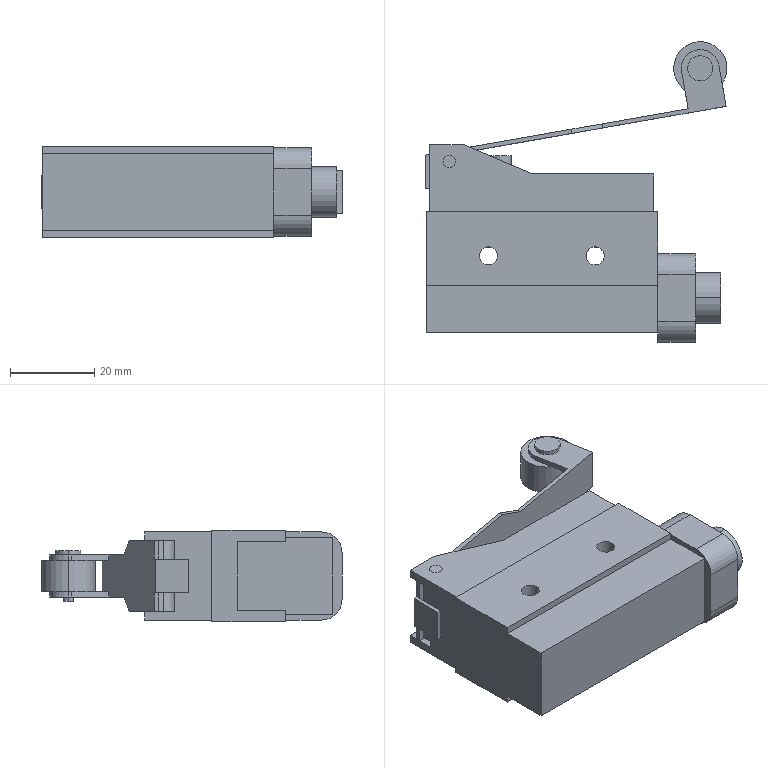Part | STEP file | 4 solids | 138 faces | box 71.855 x 71.5 x 21.7 mm | volume 42318 mm3 | plane 93 | cylinder 45 | commonest cylinder face diameters 3 x8 8 x6 10 x6 12 x6 6 x5 4.3 x4